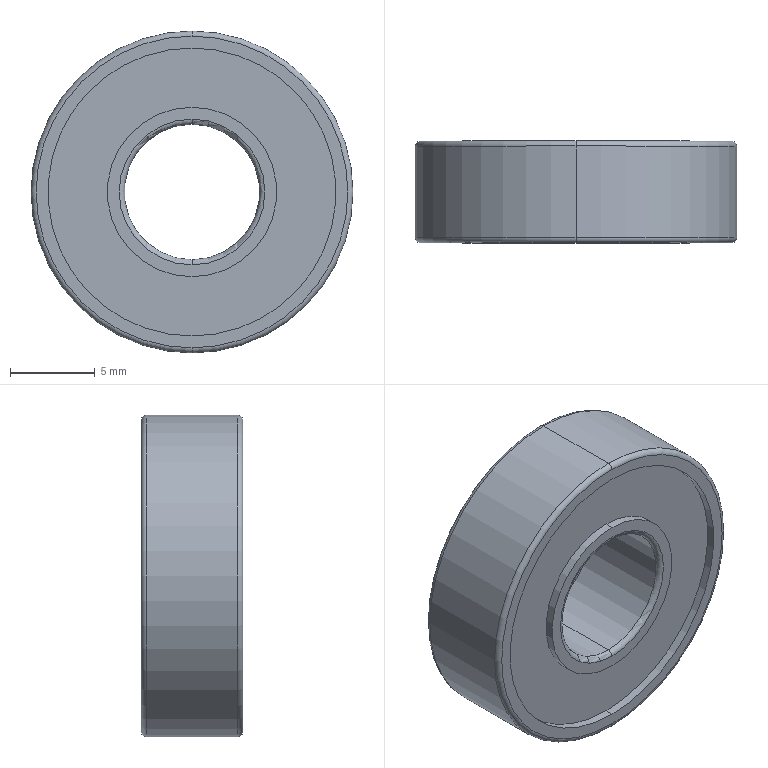Part | STEP file | Domestic miniature ball bearing NSK 698ZZ-1 | 1 solid | 26 faces | box 19 x 6 x 19 mm | volume 1248 mm3 | cylinder 12 | torus 8 | plane 6 | commonest cylinder face diameters 10 x4 17 x4 8 x2 19 x2
STEP:
#1=CARTESIAN_POINT('',(0.,22.998,-9.5));
#2=VERTEX_POINT('',#1);
#3=CARTESIAN_POINT('',(0.,22.998,9.5));
#4=VERTEX_POINT('',#3);
#5=CARTESIAN_POINT('',(0.,22.998,0.));
#6=DIRECTION('',(0.,-1.,0.));
#7=DIRECTION('',(0.,0.,1.));
#8=AXIS2_PLACEMENT_3D('',#5,#6,#7);
#9=CIRCLE('',#8,9.5);
#10=EDGE_CURVE('',#2,#4,#9,.T.);
#11=ORIENTED_EDGE('',*,*,#10,.F.);
#12=CARTESIAN_POINT('',(0.,23.298,-9.2));
#13=VERTEX_POINT('',#12);
#14=CARTESIAN_POINT('',(0.,22.998,-9.2));
#15=DIRECTION('',(1.,0.,0.));
#16=DIRECTION('',(0.,0.,-1.));
#17=AXIS2_PLACEMENT_3D('',#14,#15,#16);
#18=CIRCLE('',#17,0.3);
#19=EDGE_CURVE('',#2,#13,#18,.T.);
#20=ORIENTED_EDGE('',*,*,#19,.T.);
#21=CARTESIAN_POINT('',(0.,23.298,9.2));
#22=VERTEX_POINT('',#21);
#23=CARTESIAN_POINT('',(0.,23.298,0.));
#24=DIRECTION('',(0.,1.,0.));
#25=DIRECTION('',(0.,0.,1.));
#26=AXIS2_PLACEMENT_3D('',#23,#24,#25);
#27=CIRCLE('',#26,9.2);
#28=EDGE_CURVE('',#22,#13,#27,.T.);
#29=ORIENTED_EDGE('',*,*,#28,.F.);
#30=CARTESIAN_POINT('',(0.,22.998,9.2));
#31=DIRECTION('',(-1.,0.,0.));
#32=DIRECTION('',(0.,0.,1.));
#33=AXIS2_PLACEMENT_3D('',#30,#31,#32);
#34=CIRCLE('',#33,0.3);
#35=EDGE_CURVE('',#4,#22,#34,.T.);
#36=ORIENTED_EDGE('',*,*,#35,.F.);
#37=EDGE_LOOP('',(#11,#20,#29,#36));
#38=FACE_OUTER_BOUND('',#37,.T.);
#39=CARTESIAN_POINT('',(0.,22.998,0.));
#40=DIRECTION('',(0.,1.,0.));
#41=DIRECTION('',(0.,0.,1.));
#42=AXIS2_PLACEMENT_3D('',#39,#40,#41);
#43=TOROIDAL_SURFACE('',#42,9.2,0.3);
#44=ADVANCED_FACE('',(#38),#43,.T.);
#45=CARTESIAN_POINT('',(0.,17.598,9.5));
#46=VERTEX_POINT('',#45);
#47=CARTESIAN_POINT('',(0.,17.598,-9.5));
#48=VERTEX_POINT('',#47);
#49=CARTESIAN_POINT('',(0.,17.598,0.));
#50=DIRECTION('',(0.,1.,0.));
#51=DIRECTION('',(0.,0.,-1.));
#52=AXIS2_PLACEMENT_3D('',#49,#50,#51);
#53=CIRCLE('',#52,9.5);
#54=EDGE_CURVE('',#46,#48,#53,.T.);
#55=ORIENTED_EDGE('',*,*,#54,.F.);
#56=CARTESIAN_POINT('',(0.,17.298,9.2));
#57=VERTEX_POINT('',#56);
#58=CARTESIAN_POINT('',(0.,17.598,9.2));
#59=DIRECTION('',(1.,0.,0.));
#60=DIRECTION('',(0.,0.,-1.));
#61=AXIS2_PLACEMENT_3D('',#58,#59,#60);
#62=CIRCLE('',#61,0.3);
#63=EDGE_CURVE('',#46,#57,#62,.T.);
#64=ORIENTED_EDGE('',*,*,#63,.T.);
#65=CARTESIAN_POINT('',(0.,17.298,-9.2));
#66=VERTEX_POINT('',#65);
#67=CARTESIAN_POINT('',(0.,17.298,0.));
#68=DIRECTION('',(0.,-1.,0.));
#69=DIRECTION('',(0.,0.,-1.));
#70=AXIS2_PLACEMENT_3D('',#67,#68,#69);
#71=CIRCLE('',#70,9.2);
#72=EDGE_CURVE('',#66,#57,#71,.T.);
#73=ORIENTED_EDGE('',*,*,#72,.F.);
#74=CARTESIAN_POINT('',(0.,17.598,-9.2));
#75=DIRECTION('',(-1.,0.,0.));
#76=DIRECTION('',(0.,0.,1.));
#77=AXIS2_PLACEMENT_3D('',#74,#75,#76);
#78=CIRCLE('',#77,0.3);
#79=EDGE_CURVE('',#48,#66,#78,.T.);
#80=ORIENTED_EDGE('',*,*,#79,.F.);
#81=EDGE_LOOP('',(#55,#64,#73,#80));
#82=FACE_OUTER_BOUND('',#81,.T.);
#83=CARTESIAN_POINT('',(0.,17.598,0.));
#84=DIRECTION('',(0.,-1.,0.));
#85=DIRECTION('',(0.,0.,-1.));
#86=AXIS2_PLACEMENT_3D('',#83,#84,#85);
#87=TOROIDAL_SURFACE('',#86,9.2,0.3);
#88=ADVANCED_FACE('',(#82),#87,.T.);
#89=CARTESIAN_POINT('',(0.,23.298,-4.3));
#90=VERTEX_POINT('',#89);
#91=CARTESIAN_POINT('',(0.,23.298,4.3));
#92=VERTEX_POINT('',#91);
#93=CARTESIAN_POINT('',(0.,23.298,0.));
#94=DIRECTION('',(0.,-1.,0.));
#95=DIRECTION('',(0.,0.,1.));
#96=AXIS2_PLACEMENT_3D('',#93,#94,#95);
#97=CIRCLE('',#96,4.3);
#98=EDGE_CURVE('',#90,#92,#97,.T.);
#99=ORIENTED_EDGE('',*,*,#98,.F.);
#100=CARTESIAN_POINT('',(0.,22.998,-4.));
#101=VERTEX_POINT('',#100);
#102=CARTESIAN_POINT('',(0.,22.998,-4.3));
#103=DIRECTION('',(1.,0.,0.));
#104=DIRECTION('',(0.,0.,-1.));
#105=AXIS2_PLACEMENT_3D('',#102,#103,#104);
#106=CIRCLE('',#105,0.3);
#107=EDGE_CURVE('',#90,#101,#106,.T.);
#108=ORIENTED_EDGE('',*,*,#107,.T.);
#109=CARTESIAN_POINT('',(0.,22.998,4.));
#110=VERTEX_POINT('',#109);
#111=CARTESIAN_POINT('',(0.,22.998,0.));
#112=DIRECTION('',(0.,1.,0.));
#113=DIRECTION('',(0.,0.,1.));
#114=AXIS2_PLACEMENT_3D('',#111,#112,#113);
#115=CIRCLE('',#114,4.);
#116=EDGE_CURVE('',#110,#101,#115,.T.);
#117=ORIENTED_EDGE('',*,*,#116,.F.);
#118=CARTESIAN_POINT('',(0.,22.998,4.3));
#119=DIRECTION('',(-1.,0.,0.));
#120=DIRECTION('',(0.,0.,1.));
#121=AXIS2_PLACEMENT_3D('',#118,#119,#120);
#122=CIRCLE('',#121,0.3);
#123=EDGE_CURVE('',#92,#110,#122,.T.);
#124=ORIENTED_EDGE('',*,*,#123,.F.);
#125=EDGE_LOOP('',(#99,#108,#117,#124));
#126=FACE_OUTER_BOUND('',#125,.T.);
#127=CARTESIAN_POINT('',(0.,22.998,0.));
#128=DIRECTION('',(0.,1.,0.));
#129=DIRECTION('',(0.,0.,1.));
#130=AXIS2_PLACEMENT_3D('',#127,#128,#129);
#131=TOROIDAL_SURFACE('',#130,4.3,0.3);
#132=ADVANCED_FACE('',(#126),#131,.T.);
#133=CARTESIAN_POINT('',(0.,17.298,4.3));
#134=VERTEX_POINT('',#133);
#135=CARTESIAN_POINT('',(0.,17.298,-4.3));
#136=VERTEX_POINT('',#135);
#137=CARTESIAN_POINT('',(0.,17.298,0.));
#138=DIRECTION('',(0.,1.,0.));
#139=DIRECTION('',(0.,0.,-1.));
#140=AXIS2_PLACEMENT_3D('',#137,#138,#139);
#141=CIRCLE('',#140,4.3);
#142=EDGE_CURVE('',#134,#136,#141,.T.);
#143=ORIENTED_EDGE('',*,*,#142,.F.);
#144=CARTESIAN_POINT('',(0.,17.598,4.));
#145=VERTEX_POINT('',#144);
#146=CARTESIAN_POINT('',(0.,17.598,4.3));
#147=DIRECTION('',(1.,0.,0.));
#148=DIRECTION('',(0.,0.,-1.));
#149=AXIS2_PLACEMENT_3D('',#146,#147,#148);
#150=CIRCLE('',#149,0.3);
#151=EDGE_CURVE('',#134,#145,#150,.T.);
#152=ORIENTED_EDGE('',*,*,#151,.T.);
#153=CARTESIAN_POINT('',(0.,17.598,-4.));
#154=VERTEX_POINT('',#153);
#155=CARTESIAN_POINT('',(0.,17.598,0.));
#156=DIRECTION('',(0.,-1.,0.));
#157=DIRECTION('',(0.,0.,-1.));
#158=AXIS2_PLACEMENT_3D('',#155,#156,#157);
#159=CIRCLE('',#158,4.);
#160=EDGE_CURVE('',#154,#145,#159,.T.);
#161=ORIENTED_EDGE('',*,*,#160,.F.);
#162=CARTESIAN_POINT('',(0.,17.598,-4.3));
#163=DIRECTION('',(-1.,0.,0.));
#164=DIRECTION('',(0.,0.,1.));
#165=AXIS2_PLACEMENT_3D('',#162,#163,#164);
#166=CIRCLE('',#165,0.3);
#167=EDGE_CURVE('',#136,#154,#166,.T.);
#168=ORIENTED_EDGE('',*,*,#167,.F.);
#169=EDGE_LOOP('',(#143,#152,#161,#168));
#170=FACE_OUTER_BOUND('',#169,.T.);
#171=CARTESIAN_POINT('',(0.,17.598,0.));
#172=DIRECTION('',(0.,-1.,0.));
#173=DIRECTION('',(0.,0.,-1.));
#174=AXIS2_PLACEMENT_3D('',#171,#172,#173);
#175=TOROIDAL_SURFACE('',#174,4.3,0.3);
#176=ADVANCED_FACE('',(#170),#175,.T.);
#177=CARTESIAN_POINT('',(0.,23.298,-5.));
#178=VERTEX_POINT('',#177);
#179=CARTESIAN_POINT('',(0.,23.298,5.));
#180=VERTEX_POINT('',#179);
#181=CARTESIAN_POINT('',(0.,23.298,0.));
#182=DIRECTION('',(0.,-1.,0.));
#183=DIRECTION('',(0.,0.,-1.));
#184=AXIS2_PLACEMENT_3D('',#181,#182,#183);
#185=CIRCLE('',#184,5.);
#186=EDGE_CURVE('',#178,#180,#185,.T.);
#187=ORIENTED_EDGE('',*,*,#186,.T.);
#188=CARTESIAN_POINT('',(0.,22.798,5.));
#189=VERTEX_POINT('',#188);
#190=CARTESIAN_POINT('',(0.,0.,5.));
#191=DIRECTION('',(0.,-1.,0.));
#192=VECTOR('',#191,1000.);
#193=LINE('',#190,#192);
#194=EDGE_CURVE('',#180,#189,#193,.T.);
#195=ORIENTED_EDGE('',*,*,#194,.T.);
#196=CARTESIAN_POINT('',(0.,22.798,-5.));
#197=VERTEX_POINT('',#196);
#198=CARTESIAN_POINT('',(0.,22.798,0.));
#199=DIRECTION('',(0.,-1.,0.));
#200=DIRECTION('',(0.,0.,-1.));
#201=AXIS2_PLACEMENT_3D('',#198,#199,#200);
#202=CIRCLE('',#201,5.);
#203=EDGE_CURVE('',#197,#189,#202,.T.);
#204=ORIENTED_EDGE('',*,*,#203,.F.);
#205=CARTESIAN_POINT('',(0.,0.,-5.));
#206=DIRECTION('',(0.,-1.,0.));
#207=VECTOR('',#206,1000.);
#208=LINE('',#205,#207);
#209=EDGE_CURVE('',#178,#197,#208,.T.);
#210=ORIENTED_EDGE('',*,*,#209,.F.);
#211=EDGE_LOOP('',(#187,#195,#204,#210));
#212=FACE_OUTER_BOUND('',#211,.T.);
#213=CARTESIAN_POINT('',(0.,0.,0.));
#214=DIRECTION('',(0.,-1.,0.));
#215=DIRECTION('',(0.,0.,-1.));
#216=AXIS2_PLACEMENT_3D('',#213,#214,#215);
#217=CYLINDRICAL_SURFACE('',#216,5.);
#218=ADVANCED_FACE('',(#212),#217,.T.);
#219=CARTESIAN_POINT('',(0.,23.298,8.5));
#220=VERTEX_POINT('',#219);
#221=CARTESIAN_POINT('',(0.,23.298,-8.5));
#222=VERTEX_POINT('',#221);
#223=CARTESIAN_POINT('',(0.,23.298,0.));
#224=DIRECTION('',(0.,-1.,0.));
#225=DIRECTION('',(0.,0.,-1.));
#226=AXIS2_PLACEMENT_3D('',#223,#224,#225);
#227=CIRCLE('',#226,8.5);
#228=EDGE_CURVE('',#220,#222,#227,.T.);
#229=ORIENTED_EDGE('',*,*,#228,.F.);
#230=CARTESIAN_POINT('',(0.,22.798,8.5));
#231=VERTEX_POINT('',#230);
#232=CARTESIAN_POINT('',(0.,0.,8.5));
#233=DIRECTION('',(0.,-1.,0.));
#234=VECTOR('',#233,1000.);
#235=LINE('',#232,#234);
#236=EDGE_CURVE('',#220,#231,#235,.T.);
#237=ORIENTED_EDGE('',*,*,#236,.T.);
#238=CARTESIAN_POINT('',(0.,22.798,-8.5));
#239=VERTEX_POINT('',#238);
#240=CARTESIAN_POINT('',(0.,22.798,0.));
#241=DIRECTION('',(0.,-1.,0.));
#242=DIRECTION('',(0.,0.,-1.));
#243=AXIS2_PLACEMENT_3D('',#240,#241,#242);
#244=CIRCLE('',#243,8.5);
#245=EDGE_CURVE('',#231,#239,#244,.T.);
#246=ORIENTED_EDGE('',*,*,#245,.T.);
#247=CARTESIAN_POINT('',(0.,0.,-8.5));
#248=DIRECTION('',(0.,-1.,0.));
#249=VECTOR('',#248,1000.);
#250=LINE('',#247,#249);
#251=EDGE_CURVE('',#222,#239,#250,.T.);
#252=ORIENTED_EDGE('',*,*,#251,.F.);
#253=EDGE_LOOP('',(#229,#237,#246,#252));
#254=FACE_OUTER_BOUND('',#253,.T.);
#255=CARTESIAN_POINT('',(0.,0.,0.));
#256=DIRECTION('',(0.,-1.,0.));
#257=DIRECTION('',(0.,0.,-1.));
#258=AXIS2_PLACEMENT_3D('',#255,#256,#257);
#259=CYLINDRICAL_SURFACE('',#258,8.5);
#260=ADVANCED_FACE('',(#254),#259,.F.);
#261=ORIENTED_EDGE('',*,*,#10,.T.);
#262=CARTESIAN_POINT('',(0.,0.,9.5));
#263=DIRECTION('',(0.,-1.,0.));
#264=VECTOR('',#263,1000.);
#265=LINE('',#262,#264);
#266=EDGE_CURVE('',#4,#46,#265,.T.);
#267=ORIENTED_EDGE('',*,*,#266,.T.);
#268=ORIENTED_EDGE('',*,*,#54,.T.);
#269=CARTESIAN_POINT('',(0.,0.,-9.5));
#270=DIRECTION('',(0.,-1.,0.));
#271=VECTOR('',#270,1000.);
#272=LINE('',#269,#271);
#273=EDGE_CURVE('',#2,#48,#272,.T.);
#274=ORIENTED_EDGE('',*,*,#273,.F.);
#275=EDGE_LOOP('',(#261,#267,#268,#274));
#276=FACE_OUTER_BOUND('',#275,.T.);
#277=CARTESIAN_POINT('',(0.,0.,0.));
#278=DIRECTION('',(0.,-1.,0.));
#279=DIRECTION('',(0.,0.,-1.));
#280=AXIS2_PLACEMENT_3D('',#277,#278,#279);
#281=CYLINDRICAL_SURFACE('',#280,9.5);
#282=ADVANCED_FACE('',(#276),#281,.T.);
#283=CARTESIAN_POINT('',(0.,17.798,8.5));
#284=VERTEX_POINT('',#283);
#285=CARTESIAN_POINT('',(0.,17.798,-8.5));
#286=VERTEX_POINT('',#285);
#287=CARTESIAN_POINT('',(0.,17.798,0.));
#288=DIRECTION('',(0.,-1.,0.));
#289=DIRECTION('',(0.,0.,-1.));
#290=AXIS2_PLACEMENT_3D('',#287,#288,#289);
#291=CIRCLE('',#290,8.5);
#292=EDGE_CURVE('',#284,#286,#291,.T.);
#293=ORIENTED_EDGE('',*,*,#292,.F.);
#294=CARTESIAN_POINT('',(0.,17.298,8.5));
#295=VERTEX_POINT('',#294);
#296=CARTESIAN_POINT('',(0.,0.,8.5));
#297=DIRECTION('',(0.,-1.,0.));
#298=VECTOR('',#297,1000.);
#299=LINE('',#296,#298);
#300=EDGE_CURVE('',#284,#295,#299,.T.);
#301=ORIENTED_EDGE('',*,*,#300,.T.);
#302=CARTESIAN_POINT('',(0.,17.298,-8.5));
#303=VERTEX_POINT('',#302);
#304=CARTESIAN_POINT('',(0.,17.298,0.));
#305=DIRECTION('',(0.,-1.,0.));
#306=DIRECTION('',(0.,0.,-1.));
#307=AXIS2_PLACEMENT_3D('',#304,#305,#306);
#308=CIRCLE('',#307,8.5);
#309=EDGE_CURVE('',#295,#303,#308,.T.);
#310=ORIENTED_EDGE('',*,*,#309,.T.);
#311=CARTESIAN_POINT('',(0.,0.,-8.5));
#312=DIRECTION('',(0.,-1.,0.));
#313=VECTOR('',#312,1000.);
#314=LINE('',#311,#313);
#315=EDGE_CURVE('',#286,#303,#314,.T.);
#316=ORIENTED_EDGE('',*,*,#315,.F.);
#317=EDGE_LOOP('',(#293,#301,#310,#316));
#318=FACE_OUTER_BOUND('',#317,.T.);
#319=CARTESIAN_POINT('',(0.,0.,0.));
#320=DIRECTION('',(0.,-1.,0.));
#321=DIRECTION('',(0.,0.,-1.));
#322=AXIS2_PLACEMENT_3D('',#319,#320,#321);
#323=CYLINDRICAL_SURFACE('',#322,8.5);
#324=ADVANCED_FACE('',(#318),#323,.F.);
#325=CARTESIAN_POINT('',(0.,17.798,-5.));
#326=VERTEX_POINT('',#325);
#327=CARTESIAN_POINT('',(0.,17.798,5.));
#328=VERTEX_POINT('',#327);
#329=CARTESIAN_POINT('',(0.,17.798,0.));
#330=DIRECTION('',(0.,-1.,0.));
#331=DIRECTION('',(0.,0.,-1.));
#332=AXIS2_PLACEMENT_3D('',#329,#330,#331);
#333=CIRCLE('',#332,5.);
#334=EDGE_CURVE('',#326,#328,#333,.T.);
#335=ORIENTED_EDGE('',*,*,#334,.T.);
#336=CARTESIAN_POINT('',(0.,17.298,5.));
#337=VERTEX_POINT('',#336);
#338=CARTESIAN_POINT('',(0.,0.,5.));
#339=DIRECTION('',(0.,-1.,0.));
#340=VECTOR('',#339,1000.);
#341=LINE('',#338,#340);
#342=EDGE_CURVE('',#328,#337,#341,.T.);
#343=ORIENTED_EDGE('',*,*,#342,.T.);
#344=CARTESIAN_POINT('',(0.,17.298,-5.));
#345=VERTEX_POINT('',#344);
#346=CARTESIAN_POINT('',(0.,17.298,0.));
#347=DIRECTION('',(0.,-1.,0.));
#348=DIRECTION('',(0.,0.,-1.));
#349=AXIS2_PLACEMENT_3D('',#346,#347,#348);
#350=CIRCLE('',#349,5.);
#351=EDGE_CURVE('',#345,#337,#350,.T.);
#352=ORIENTED_EDGE('',*,*,#351,.F.);
#353=CARTESIAN_POINT('',(0.,0.,-5.));
#354=DIRECTION('',(0.,-1.,0.));
#355=VECTOR('',#354,1000.);
#356=LINE('',#353,#355);
#357=EDGE_CURVE('',#326,#345,#356,.T.);
#358=ORIENTED_EDGE('',*,*,#357,.F.);
#359=EDGE_LOOP('',(#335,#343,#352,#358));
#360=FACE_OUTER_BOUND('',#359,.T.);
#361=CARTESIAN_POINT('',(0.,0.,0.));
#362=DIRECTION('',(0.,-1.,0.));
#363=DIRECTION('',(0.,0.,-1.));
#364=AXIS2_PLACEMENT_3D('',#361,#362,#363);
#365=CYLINDRICAL_SURFACE('',#364,5.);
#366=ADVANCED_FACE('',(#360),#365,.T.);
#367=CARTESIAN_POINT('',(0.,22.998,0.));
#368=DIRECTION('',(0.,1.,0.));
#369=DIRECTION('',(0.,0.,1.));
#370=AXIS2_PLACEMENT_3D('',#367,#368,#369);
#371=CIRCLE('',#370,4.);
#372=EDGE_CURVE('',#101,#110,#371,.T.);
#373=ORIENTED_EDGE('',*,*,#372,.T.);
#374=CARTESIAN_POINT('',(0.,0.,4.));
#375=DIRECTION('',(0.,-1.,0.));
#376=VECTOR('',#375,1000.);
#377=LINE('',#374,#376);
#378=EDGE_CURVE('',#110,#145,#377,.T.);
#379=ORIENTED_EDGE('',*,*,#378,.T.);
#380=CARTESIAN_POINT('',(0.,17.598,0.));
#381=DIRECTION('',(0.,-1.,0.));
#382=DIRECTION('',(0.,0.,-1.));
#383=AXIS2_PLACEMENT_3D('',#380,#381,#382);
#384=CIRCLE('',#383,4.);
#385=EDGE_CURVE('',#145,#154,#384,.T.);
#386=ORIENTED_EDGE('',*,*,#385,.T.);
#387=CARTESIAN_POINT('',(0.,0.,-4.));
#388=DIRECTION('',(0.,-1.,0.));
#389=VECTOR('',#388,1000.);
#390=LINE('',#387,#389);
#391=EDGE_CURVE('',#101,#154,#390,.T.);
#392=ORIENTED_EDGE('',*,*,#391,.F.);
#393=EDGE_LOOP('',(#373,#379,#386,#392));
#394=FACE_OUTER_BOUND('',#393,.T.);
#395=CARTESIAN_POINT('',(0.,0.,0.));
#396=DIRECTION('',(0.,-1.,0.));
#397=DIRECTION('',(0.,0.,-1.));
#398=AXIS2_PLACEMENT_3D('',#395,#396,#397);
#399=CYLINDRICAL_SURFACE('',#398,4.);
#400=ADVANCED_FACE('',(#394),#399,.F.);
#401=CARTESIAN_POINT('',(0.,23.298,0.));
#402=DIRECTION('',(0.,-1.,0.));
#403=DIRECTION('',(0.,0.,1.));
#404=AXIS2_PLACEMENT_3D('',#401,#402,#403);
#405=CIRCLE('',#404,4.3);
#406=EDGE_CURVE('',#92,#90,#405,.T.);
#407=ORIENTED_EDGE('',*,*,#406,.T.);
#408=ORIENTED_EDGE('',*,*,#98,.T.);
#409=EDGE_LOOP('',(#407,#408));
#410=FACE_BOUND('',#409,.T.);
#411=ORIENTED_EDGE('',*,*,#186,.F.);
#412=CARTESIAN_POINT('',(0.,23.298,0.));
#413=DIRECTION('',(0.,-1.,0.));
#414=DIRECTION('',(0.,0.,-1.));
#415=AXIS2_PLACEMENT_3D('',#412,#413,#414);
#416=CIRCLE('',#415,5.);
#417=EDGE_CURVE('',#180,#178,#416,.T.);
#418=ORIENTED_EDGE('',*,*,#417,.F.);
#419=EDGE_LOOP('',(#411,#418));
#420=FACE_OUTER_BOUND('',#419,.T.);
#421=CARTESIAN_POINT('',(5.,23.298,0.));
#422=DIRECTION('',(0.,1.,0.));
#423=DIRECTION('',(0.,0.,1.));
#424=AXIS2_PLACEMENT_3D('',#421,#422,#423);
#425=PLANE('',#424);
#426=ADVANCED_FACE('',(#410,#420),#425,.T.);
#427=ORIENTED_EDGE('',*,*,#378,.F.);
#428=ORIENTED_EDGE('',*,*,#116,.T.);
#429=ORIENTED_EDGE('',*,*,#391,.T.);
#430=ORIENTED_EDGE('',*,*,#160,.T.);
#431=EDGE_LOOP('',(#427,#428,#429,#430));
#432=FACE_OUTER_BOUND('',#431,.T.);
#433=CARTESIAN_POINT('',(0.,0.,0.));
#434=DIRECTION('',(0.,-1.,0.));
#435=DIRECTION('',(0.,0.,-1.));
#436=AXIS2_PLACEMENT_3D('',#433,#434,#435);
#437=CYLINDRICAL_SURFACE('',#436,4.);
#438=ADVANCED_FACE('',(#432),#437,.F.);
#439=CARTESIAN_POINT('',(0.,17.298,0.));
#440=DIRECTION('',(0.,1.,0.));
#441=DIRECTION('',(0.,0.,-1.));
#442=AXIS2_PLACEMENT_3D('',#439,#440,#441);
#443=CIRCLE('',#442,4.3);
#444=EDGE_CURVE('',#136,#134,#443,.T.);
#445=ORIENTED_EDGE('',*,*,#444,.T.);
#446=ORIENTED_EDGE('',*,*,#142,.T.);
#447=EDGE_LOOP('',(#445,#446));
#448=FACE_BOUND('',#447,.T.);
#449=ORIENTED_EDGE('',*,*,#351,.T.);
#450=CARTESIAN_POINT('',(0.,17.298,0.));
#451=DIRECTION('',(0.,-1.,0.));
#452=DIRECTION('',(0.,0.,-1.));
#453=AXIS2_PLACEMENT_3D('',#450,#451,#452);
#454=CIRCLE('',#453,5.);
#455=EDGE_CURVE('',#337,#345,#454,.T.);
#456=ORIENTED_EDGE('',*,*,#455,.T.);
#457=EDGE_LOOP('',(#449,#456));
#458=FACE_OUTER_BOUND('',#457,.T.);
#459=CARTESIAN_POINT('',(4.,17.298,0.));
#460=DIRECTION('',(0.,-1.,0.));
#461=DIRECTION('',(0.,0.,-1.));
#462=AXIS2_PLACEMENT_3D('',#459,#460,#461);
#463=PLANE('',#462);
#464=ADVANCED_FACE('',(#448,#458),#463,.T.);
#465=ORIENTED_EDGE('',*,*,#342,.F.);
#466=CARTESIAN_POINT('',(0.,17.798,0.));
#467=DIRECTION('',(0.,-1.,0.));
#468=DIRECTION('',(0.,0.,-1.));
#469=AXIS2_PLACEMENT_3D('',#466,#467,#468);
#470=CIRCLE('',#469,5.);
#471=EDGE_CURVE('',#328,#326,#470,.T.);
#472=ORIENTED_EDGE('',*,*,#471,.T.);
#473=ORIENTED_EDGE('',*,*,#357,.T.);
#474=ORIENTED_EDGE('',*,*,#455,.F.);
#475=EDGE_LOOP('',(#465,#472,#473,#474));
#476=FACE_OUTER_BOUND('',#475,.T.);
#477=CARTESIAN_POINT('',(0.,0.,0.));
#478=DIRECTION('',(0.,-1.,0.));
#479=DIRECTION('',(0.,0.,-1.));
#480=AXIS2_PLACEMENT_3D('',#477,#478,#479);
#481=CYLINDRICAL_SURFACE('',#480,5.);
#482=ADVANCED_FACE('',(#476),#481,.T.);
#483=CARTESIAN_POINT('',(0.,17.798,0.));
#484=DIRECTION('',(0.,-1.,0.));
#485=DIRECTION('',(0.,0.,-1.));
#486=AXIS2_PLACEMENT_3D('',#483,#484,#485);
#487=CIRCLE('',#486,8.5);
#488=EDGE_CURVE('',#286,#284,#487,.T.);
#489=ORIENTED_EDGE('',*,*,#488,.T.);
#490=ORIENTED_EDGE('',*,*,#292,.T.);
#491=EDGE_LOOP('',(#489,#490));
#492=FACE_OUTER_BOUND('',#491,.T.);
#493=ORIENTED_EDGE('',*,*,#334,.F.);
#494=ORIENTED_EDGE('',*,*,#471,.F.);
#495=EDGE_LOOP('',(#493,#494));
#496=FACE_BOUND('',#495,.T.);
#497=CARTESIAN_POINT('',(5.,17.798,0.));
#498=DIRECTION('',(0.,-1.,0.));
#499=DIRECTION('',(0.,0.,-1.));
#500=AXIS2_PLACEMENT_3D('',#497,#498,#499);
#501=PLANE('',#500);
#502=ADVANCED_FACE('',(#492,#496),#501,.T.);
#503=ORIENTED_EDGE('',*,*,#300,.F.);
#504=ORIENTED_EDGE('',*,*,#488,.F.);
#505=ORIENTED_EDGE('',*,*,#315,.T.);
#506=CARTESIAN_POINT('',(0.,17.298,0.));
#507=DIRECTION('',(0.,-1.,0.));
#508=DIRECTION('',(0.,0.,-1.));
#509=AXIS2_PLACEMENT_3D('',#506,#507,#508);
#510=CIRCLE('',#509,8.5);
#511=EDGE_CURVE('',#303,#295,#510,.T.);
#512=ORIENTED_EDGE('',*,*,#511,.T.);
#513=EDGE_LOOP('',(#503,#504,#505,#512));
#514=FACE_OUTER_BOUND('',#513,.T.);
#515=CARTESIAN_POINT('',(0.,0.,0.));
#516=DIRECTION('',(0.,-1.,0.));
#517=DIRECTION('',(0.,0.,-1.));
#518=AXIS2_PLACEMENT_3D('',#515,#516,#517);
#519=CYLINDRICAL_SURFACE('',#518,8.5);
#520=ADVANCED_FACE('',(#514),#519,.F.);
#521=ORIENTED_EDGE('',*,*,#72,.T.);
#522=CARTESIAN_POINT('',(0.,17.298,0.));
#523=DIRECTION('',(0.,-1.,0.));
#524=DIRECTION('',(0.,0.,-1.));
#525=AXIS2_PLACEMENT_3D('',#522,#523,#524);
#526=CIRCLE('',#525,9.2);
#527=EDGE_CURVE('',#57,#66,#526,.T.);
#528=ORIENTED_EDGE('',*,*,#527,.T.);
#529=EDGE_LOOP('',(#521,#528));
#530=FACE_OUTER_BOUND('',#529,.T.);
#531=ORIENTED_EDGE('',*,*,#511,.F.);
#532=ORIENTED_EDGE('',*,*,#309,.F.);
#533=EDGE_LOOP('',(#531,#532));
#534=FACE_BOUND('',#533,.T.);
#535=CARTESIAN_POINT('',(8.5,17.298,0.));
#536=DIRECTION('',(0.,-1.,0.));
#537=DIRECTION('',(0.,0.,-1.));
#538=AXIS2_PLACEMENT_3D('',#535,#536,#537);
#539=PLANE('',#538);
#540=ADVANCED_FACE('',(#530,#534),#539,.T.);
#541=ORIENTED_EDGE('',*,*,#266,.F.);
#542=CARTESIAN_POINT('',(0.,22.998,0.));
#543=DIRECTION('',(0.,-1.,0.));
#544=DIRECTION('',(0.,0.,1.));
#545=AXIS2_PLACEMENT_3D('',#542,#543,#544);
#546=CIRCLE('',#545,9.5);
#547=EDGE_CURVE('',#4,#2,#546,.T.);
#548=ORIENTED_EDGE('',*,*,#547,.T.);
#549=ORIENTED_EDGE('',*,*,#273,.T.);
#550=CARTESIAN_POINT('',(0.,17.598,0.));
#551=DIRECTION('',(0.,1.,0.));
#552=DIRECTION('',(0.,0.,-1.));
#553=AXIS2_PLACEMENT_3D('',#550,#551,#552);
#554=CIRCLE('',#553,9.5);
#555=EDGE_CURVE('',#48,#46,#554,.T.);
#556=ORIENTED_EDGE('',*,*,#555,.T.);
#557=EDGE_LOOP('',(#541,#548,#549,#556));
#558=FACE_OUTER_BOUND('',#557,.T.);
#559=CARTESIAN_POINT('',(0.,0.,0.));
#560=DIRECTION('',(0.,-1.,0.));
#561=DIRECTION('',(0.,0.,-1.));
#562=AXIS2_PLACEMENT_3D('',#559,#560,#561);
#563=CYLINDRICAL_SURFACE('',#562,9.5);
#564=ADVANCED_FACE('',(#558),#563,.T.);
#565=ORIENTED_EDGE('',*,*,#28,.T.);
#566=CARTESIAN_POINT('',(0.,23.298,0.));
#567=DIRECTION('',(0.,1.,0.));
#568=DIRECTION('',(0.,0.,1.));
#569=AXIS2_PLACEMENT_3D('',#566,#567,#568);
#570=CIRCLE('',#569,9.2);
#571=EDGE_CURVE('',#13,#22,#570,.T.);
#572=ORIENTED_EDGE('',*,*,#571,.T.);
#573=EDGE_LOOP('',(#565,#572));
#574=FACE_OUTER_BOUND('',#573,.T.);
#575=CARTESIAN_POINT('',(0.,23.298,0.));
#576=DIRECTION('',(0.,-1.,0.));
#577=DIRECTION('',(0.,0.,-1.));
#578=AXIS2_PLACEMENT_3D('',#575,#576,#577);
#579=CIRCLE('',#578,8.5);
#580=EDGE_CURVE('',#222,#220,#579,.T.);
#581=ORIENTED_EDGE('',*,*,#580,.T.);
#582=ORIENTED_EDGE('',*,*,#228,.T.);
#583=EDGE_LOOP('',(#581,#582));
#584=FACE_BOUND('',#583,.T.);
#585=CARTESIAN_POINT('',(9.5,23.298,0.));
#586=DIRECTION('',(0.,1.,0.));
#587=DIRECTION('',(0.,0.,1.));
#588=AXIS2_PLACEMENT_3D('',#585,#586,#587);
#589=PLANE('',#588);
#590=ADVANCED_FACE('',(#574,#584),#589,.T.);
#591=ORIENTED_EDGE('',*,*,#236,.F.);
#592=ORIENTED_EDGE('',*,*,#580,.F.);
#593=ORIENTED_EDGE('',*,*,#251,.T.);
#594=CARTESIAN_POINT('',(0.,22.798,0.));
#595=DIRECTION('',(0.,-1.,0.));
#596=DIRECTION('',(0.,0.,-1.));
#597=AXIS2_PLACEMENT_3D('',#594,#595,#596);
#598=CIRCLE('',#597,8.5);
#599=EDGE_CURVE('',#239,#231,#598,.T.);
#600=ORIENTED_EDGE('',*,*,#599,.T.);
#601=EDGE_LOOP('',(#591,#592,#593,#600));
#602=FACE_OUTER_BOUND('',#601,.T.);
#603=CARTESIAN_POINT('',(0.,0.,0.));
#604=DIRECTION('',(0.,-1.,0.));
#605=DIRECTION('',(0.,0.,-1.));
#606=AXIS2_PLACEMENT_3D('',#603,#604,#605);
#607=CYLINDRICAL_SURFACE('',#606,8.5);
#608=ADVANCED_FACE('',(#602),#607,.F.);
#609=ORIENTED_EDGE('',*,*,#203,.T.);
#610=CARTESIAN_POINT('',(0.,22.798,0.));
#611=DIRECTION('',(0.,-1.,0.));
#612=DIRECTION('',(0.,0.,-1.));
#613=AXIS2_PLACEMENT_3D('',#610,#611,#612);
#614=CIRCLE('',#613,5.);
#615=EDGE_CURVE('',#189,#197,#614,.T.);
#616=ORIENTED_EDGE('',*,*,#615,.T.);
#617=EDGE_LOOP('',(#609,#616));
#618=FACE_BOUND('',#617,.T.);
#619=ORIENTED_EDGE('',*,*,#599,.F.);
#620=ORIENTED_EDGE('',*,*,#245,.F.);
#621=EDGE_LOOP('',(#619,#620));
#622=FACE_OUTER_BOUND('',#621,.T.);
#623=CARTESIAN_POINT('',(8.5,22.798,0.));
#624=DIRECTION('',(0.,1.,0.));
#625=DIRECTION('',(0.,0.,1.));
#626=AXIS2_PLACEMENT_3D('',#623,#624,#625);
#627=PLANE('',#626);
#628=ADVANCED_FACE('',(#618,#622),#627,.T.);
#629=ORIENTED_EDGE('',*,*,#194,.F.);
#630=ORIENTED_EDGE('',*,*,#417,.T.);
#631=ORIENTED_EDGE('',*,*,#209,.T.);
#632=ORIENTED_EDGE('',*,*,#615,.F.);
#633=EDGE_LOOP('',(#629,#630,#631,#632));
#634=FACE_OUTER_BOUND('',#633,.T.);
#635=CARTESIAN_POINT('',(0.,0.,0.));
#636=DIRECTION('',(0.,-1.,0.));
#637=DIRECTION('',(0.,0.,-1.));
#638=AXIS2_PLACEMENT_3D('',#635,#636,#637);
#639=CYLINDRICAL_SURFACE('',#638,5.);
#640=ADVANCED_FACE('',(#634),#639,.T.);
#641=ORIENTED_EDGE('',*,*,#151,.F.);
#642=ORIENTED_EDGE('',*,*,#444,.F.);
#643=ORIENTED_EDGE('',*,*,#167,.T.);
#644=ORIENTED_EDGE('',*,*,#385,.F.);
#645=EDGE_LOOP('',(#641,#642,#643,#644));
#646=FACE_OUTER_BOUND('',#645,.T.);
#647=CARTESIAN_POINT('',(0.,17.598,0.));
#648=DIRECTION('',(0.,-1.,0.));
#649=DIRECTION('',(0.,0.,-1.));
#650=AXIS2_PLACEMENT_3D('',#647,#648,#649);
#651=TOROIDAL_SURFACE('',#650,4.3,0.3);
#652=ADVANCED_FACE('',(#646),#651,.T.);
#653=ORIENTED_EDGE('',*,*,#107,.F.);
#654=ORIENTED_EDGE('',*,*,#406,.F.);
#655=ORIENTED_EDGE('',*,*,#123,.T.);
#656=ORIENTED_EDGE('',*,*,#372,.F.);
#657=EDGE_LOOP('',(#653,#654,#655,#656));
#658=FACE_OUTER_BOUND('',#657,.T.);
#659=CARTESIAN_POINT('',(0.,22.998,0.));
#660=DIRECTION('',(0.,1.,0.));
#661=DIRECTION('',(0.,0.,1.));
#662=AXIS2_PLACEMENT_3D('',#659,#660,#661);
#663=TOROIDAL_SURFACE('',#662,4.3,0.3);
#664=ADVANCED_FACE('',(#658),#663,.T.);
#665=ORIENTED_EDGE('',*,*,#63,.F.);
#666=ORIENTED_EDGE('',*,*,#555,.F.);
#667=ORIENTED_EDGE('',*,*,#79,.T.);
#668=ORIENTED_EDGE('',*,*,#527,.F.);
#669=EDGE_LOOP('',(#665,#666,#667,#668));
#670=FACE_OUTER_BOUND('',#669,.T.);
#671=CARTESIAN_POINT('',(0.,17.598,0.));
#672=DIRECTION('',(0.,-1.,0.));
#673=DIRECTION('',(0.,0.,-1.));
#674=AXIS2_PLACEMENT_3D('',#671,#672,#673);
#675=TOROIDAL_SURFACE('',#674,9.2,0.3);
#676=ADVANCED_FACE('',(#670),#675,.T.);
#677=ORIENTED_EDGE('',*,*,#19,.F.);
#678=ORIENTED_EDGE('',*,*,#547,.F.);
#679=ORIENTED_EDGE('',*,*,#35,.T.);
#680=ORIENTED_EDGE('',*,*,#571,.F.);
#681=EDGE_LOOP('',(#677,#678,#679,#680));
#682=FACE_OUTER_BOUND('',#681,.T.);
#683=CARTESIAN_POINT('',(0.,22.998,0.));
#684=DIRECTION('',(0.,1.,0.));
#685=DIRECTION('',(0.,0.,1.));
#686=AXIS2_PLACEMENT_3D('',#683,#684,#685);
#687=TOROIDAL_SURFACE('',#686,9.2,0.3);
#688=ADVANCED_FACE('',(#682),#687,.T.);
#689=CLOSED_SHELL('',(#44,#88,#132,#176,#218,#260,#282,#324,#366,#400,#426,#438,#464,#482,#502,#520,#540,#564,#590,#608,#628,#640,#652,#664,#676,#688));
#690=MANIFOLD_SOLID_BREP('',#689);
#691=CARTESIAN_POINT('',(0.,0.,0.));
#692=DIRECTION('',(0.,0.,1.));
#693=DIRECTION('',(1.,0.,0.));
#694=AXIS2_PLACEMENT_3D('',#691,#692,#693);
#695=(LENGTH_UNIT()NAMED_UNIT(*)SI_UNIT(.MILLI.,.METRE.));
#696=UNCERTAINTY_MEASURE_WITH_UNIT(LENGTH_MEASURE(0.00001),#695,'','');
#697=(NAMED_UNIT(*)PLANE_ANGLE_UNIT()SI_UNIT($,.RADIAN.));
#698=(NAMED_UNIT(*)SI_UNIT($,.STERADIAN.)SOLID_ANGLE_UNIT());
#699=(GEOMETRIC_REPRESENTATION_CONTEXT(3)GLOBAL_UNCERTAINTY_ASSIGNED_CONTEXT((#696))GLOBAL_UNIT_ASSIGNED_CONTEXT((#695,#697,#698))REPRESENTATION_CONTEXT('',''));
#700=ADVANCED_BREP_SHAPE_REPRESENTATION('',(#690,#694),#699);